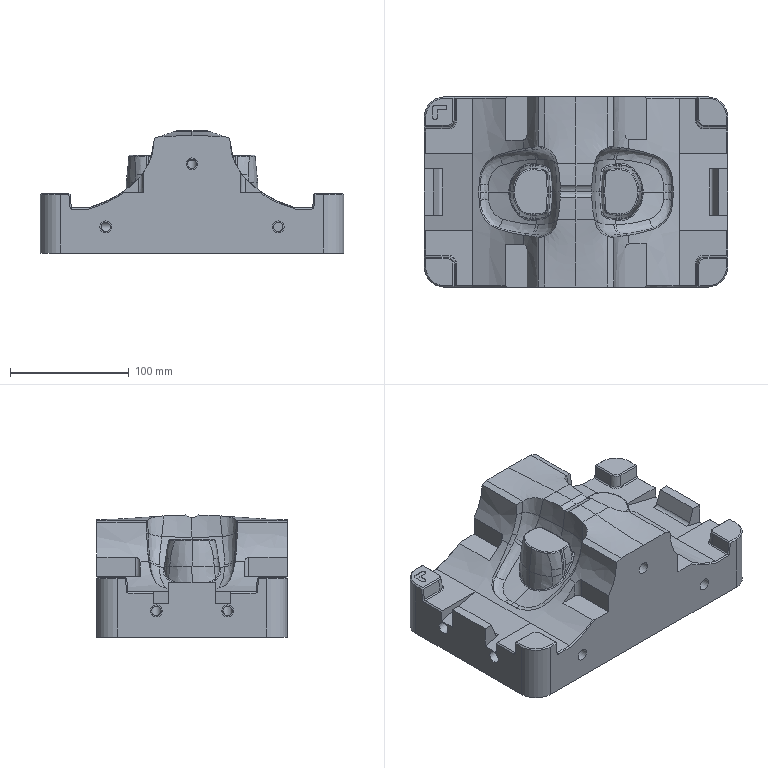NC program | NX | posted with a generic post | part box 255 x 160 x 102.619 mm
Lines 47642 to 48611 of 55104:
(ZLEVEL_PROFILE_2 , TOOL : BB6R3)
N95222 M6
N95224 G54
N95226 G17 G0 G90 X-1.967 Y96.474 S3000 M3
N95228 G43 Z51. H0
N95230 Z46.4
N95232 G94 G1 Z45.9 F1800.
N95234 X-0.764
N95236 X-0.767 Y99.474
N95238 G2 X0.026 Y100.269 R0.794
N95240 G1 X7.545
N95242 G2 X8.35 Y99.475 R0.8
N95244 G1 Y60.528
N95246 G2 X7.545 Y59.735 R0.8
N95248 G1 X0.026
N95250 G2 X-0.767 Y60.529 R0.794
N95252 G1 X-0.935 Z45.85
N95254 X-1.075 Z45.801
N95256 G3 X0.026 Y59.426 R1.102
N95258 G1 X7.545
N95260 G3 X8.659 Y60.528 R1.108
N95262 G1 Y99.475
N95264 G3 X7.545 Y100.577 R1.108
N95266 G1 X0.026
N95268 G3 X-1.075 Y99.474 R1.102
N95270 G1 X-1.197 Y99.475 Z45.751
N95272 X-1.306 Y99.476 Z45.701
N95274 G2 X0.026 Y100.807 R1.332
N95276 G1 X7.545
N95278 G2 X8.889 Y99.475 R1.338
N95280 G1 Y60.528
N95282 G2 X7.545 Y59.196 R1.338
N95284 G1 X0.026
N95286 G2 X-1.306 Y60.527 R1.332
N95288 G1 X-1.404 Z45.651
N95290 X-1.495 Z45.601
N95292 G3 X0.026 Y59.007 R1.52
N95294 G1 X7.545
N95296 G3 X9.078 Y60.528 R1.527
N95298 G1 Y99.475
N95300 G3 X7.545 Y100.996 R1.527
N95302 G1 X0.026
N95304 G3 X-1.495 Y99.476 R1.52
N95306 G1 X-1.578 Z45.551
N95308 X-1.656 Z45.502
N95310 G2 X0.026 Y101.158 R1.682
N95312 G1 X7.545
N95314 G2 X9.24 Y99.475 R1.689
N95316 G1 Y60.528
N95318 G2 X7.545 Y58.846 R1.689
N95320 G1 X0.026
N95322 G2 X-1.656 Y60.527 R1.682
N95324 G1 X-1.729 Z45.452
N95326 X-1.798 Z45.402
N95328 G3 X0.026 Y58.704 R1.823
N95330 G1 X7.545
N95332 G3 X9.381 Y60.528 R1.83
N95334 G1 Y99.475
N95336 G3 X7.545 Y101.299 R1.83
N95338 G1 X0.026
N95340 G3 X-1.798 Y99.476 R1.823
N95342 G1 X-1.924 Y99.46 Z45.302
N95344 G2 X0.026 Y101.425 R1.957
N95346 G1 X7.545
N95348 G2 X9.507 Y99.475 R1.956
N95350 G1 Y60.528
N95352 G2 X7.545 Y58.578 R1.956
N95354 G1 X0.026
N95356 G2 X-1.924 Y60.543 R1.957
N95358 G1 X-2.037 Z45.202
N95360 G3 X0.026 Y58.465 R2.071
N95362 G1 X7.545
N95364 G3 X9.62 Y60.528 R2.07
N95366 G1 Y99.475
N95368 G3 X7.545 Y101.539 R2.07
N95370 G1 X0.026
N95372 G3 X-2.037 Y99.46 R2.071
N95374 G1 X-2.14 Z45.103
N95376 G2 X0.026 Y101.641 R2.173
N95378 G1 X7.545
N95380 G2 X9.723 Y99.475 R2.172
N95382 G1 Y60.528
N95384 G2 X7.545 Y58.362 R2.172
N95386 G1 X0.026
N95388 G2 X-2.14 Y60.543 R2.173
N95390 G1 X-2.233 Z45.003
N95392 G3 X0.026 Y58.268 R2.267
N95394 G1 X7.545
N95396 G3 X9.817 Y60.528 R2.266
N95398 G1 Y99.475
N95400 G3 X7.545 Y101.735 R2.266
N95402 G1 X0.026
N95404 G3 X-2.233 Y99.46 R2.267
N95406 G1 X-2.319 Z44.903
N95408 G2 X0.026 Y101.82 R2.352
N95410 G1 X7.545
N95412 G2 X9.902 Y99.475 R2.352
N95414 G1 Y60.528
N95416 G2 X7.545 Y58.183 R2.352
N95418 G1 X0.026
N95420 G2 X-2.319 Y60.543 R2.352
N95422 G1 X-2.397 Z44.804
N95424 G3 X0.026 Y58.104 R2.431
N95426 G1 X7.545
N95428 G3 X9.981 Y60.528 R2.43
N95430 G1 Y99.475
N95432 G3 X7.545 Y101.899 R2.43
N95434 G1 X0.026
N95436 G3 X-2.397 Y99.46 R2.431
N95438 G1 X-2.469 Y99.497 Z44.704
N95440 G2 X0.062 Y101.971 R2.503
N95442 G1 X7.574
N95444 G2 X10.053 Y99.475 R2.487
N95446 G1 Y60.528
N95448 G2 X7.59 Y58.032 R2.479
N95450 G1 X0.062
N95452 G2 X-2.469 Y60.506 R2.503
N95454 G1 X-2.535 Z44.604
N95456 G3 X0. Y57.967 R2.537
N95458 G1 X7.592
N95460 G3 X10.119 Y60.528 R2.544
N95462 G1 Y99.475
N95464 G3 X7.559 Y102.037 R2.561
N95466 G1 X-0.001
N95468 G3 X-2.535 Y99.497 R2.537
N95470 G1 X-2.595 Y99.498 Z44.505
N95472 G2 X0.021 Y102.097 R2.608
N95474 G1 X7.583
N95476 G2 X10.179 Y99.475 R2.609
N95478 G1 Y60.528
N95480 G2 X7.592 Y57.906 R2.605
N95482 G1 X0.021
N95484 G2 X-2.595 Y60.505 R2.608
N95486 G1 X-2.651 Y60.504 Z44.405
N95488 G3 X0.009 Y57.851 R2.656
N95490 G1 X7.585
N95492 G3 X10.234 Y60.528 R2.664
N95494 G1 Y99.475
N95496 G3 X7.578 Y102.152 R2.667
N95498 G1 X0.009
N95500 G3 X-2.651 Y99.499 R2.656
N95502 G1 X-2.701 Y99.5 Z44.305
N95504 G2 X0.001 Y102.203 R2.703
N95506 G1 X7.578
N95508 G2 X10.196 Y100.175 R2.726
N95510 G1 X10.267 Y99.507
N95512 X10.285 Y99.475
N95514 Y60.528
N95516 X10.267 Y60.496
N95518 X10.196 Y59.828
N95520 G2 X7.602 Y57.8 R2.727
N95522 G1 X0.001
N95524 G2 X-2.701 Y60.503 R2.703
N95526 G1 X-2.747 Z44.205
N95528 G3 X0.005 Y57.754 R2.75
N95530 G1 X7.583
N95532 G3 X10.234 Y59.828 R2.741
N95534 G1 X10.31 Y60.496
N95536 X10.331 Y60.528
N95538 Y99.475
N95540 X10.31 Y99.507
N95542 X10.234 Y100.175
N95544 G3 X7.582 Y102.249 R2.741
N95546 G1 X0.
N95548 G3 X-2.747 Y99.5 R2.748
N95550 G1 X-2.789 Y99.501 Z44.106
N95552 G2 X-0.002 Y102.29 R2.788
N95554 G1 X7.54
N95556 G2 X10.353 Y99.507 R2.774
N95558 G1 X10.372 Y99.475
N95560 Y60.528
N95562 X10.353 Y60.496
N95564 G2 X7.583 Y57.713 R2.773
N95566 G1 X0.01
N95568 G2 X-2.789 Y60.502 R2.794
N95570 G1 X-2.826 Z44.006
N95572 G3 X0.003 Y57.675 R2.828
N95574 G1 X7.58
N95576 G3 X10.41 Y60.502 R2.847
N95578 G1 Y99.502
N95580 G3 X7.553 Y102.328 R2.847
N95582 G1 X0.003
N95584 G3 X-2.826 Y99.501 R2.828
N95586 G1 X-2.86 Y99.47 Z43.906
N95588 G2 X0.012 Y102.361 R2.882
N95590 G1 X7.578
N95592 G2 X10.446 Y99.502 R2.89
N95594 G1 Y60.502
N95596 G2 X7.578 Y57.642 R2.89
N95598 G1 X0.012
N95600 G2 X-2.86 Y60.534 R2.882
N95602 G1 X-2.89 Y60.533 Z43.807
N95604 G3 X0.025 Y57.612 R2.918
N95606 G1 X7.554
N95608 G3 X10.482 Y60.502 R2.909
N95610 G1 Y99.502
N95612 G3 X7.549 Y102.391 R2.912
N95614 G1 X0.025
N95616 G3 X-2.89 Y99.47 R2.918
N95618 G1 X-2.916 Z43.707
N95620 G2 X-0.001 Y102.417 R2.931
N95622 G1 X7.581
N95624 G2 X10.519 Y99.502 R2.965
N95626 G1 Y60.502
N95628 G2 X7.528 Y57.586 R2.953
N95630 G1 X0.02
N95632 G2 X-2.916 Y60.533 R2.941
N95634 G1 X-2.938 Y60.532 Z43.607
N95636 G3 X0.019 Y57.564 R2.963
N95638 G1 X7.57
N95640 G3 X10.555 Y60.502 R2.996
N95642 G1 Y99.502
N95644 G3 X7.559 Y102.439 R2.996
N95646 G1 X0.019
N95648 G3 X-2.938 Y99.471 R2.963
N95650 G1 X-2.957 Z43.508
N95652 G2 X0.001 Y102.458 R2.98
N95654 G1 X7.54
N95656 G2 X10.591 Y99.502 R3.025
N95658 G1 Y60.502
N95660 G2 X7.552 Y57.545 R3.025
N95662 G1 X0.001
N95664 G2 X-2.957 Y60.532 R2.98
N95666 G1 X-2.972 Z43.408
N95668 G3 X0.028 Y57.529 R3.018
N95670 G1 X7.579
N95672 G3 X10.628 Y60.502 R3.052
N95674 G1 Y99.502
N95676 G3 X7.567 Y102.474 R3.053
N95678 G1 X0.028
N95680 G3 X-2.972 Y99.471 R3.001
N95682 G1 X-2.984 Z43.308
N95684 G2 X0.016 Y102.486 R3.016
N95686 G1 X7.555
N95688 G2 X9.976 Y101.361 R3.218
N95690 X10.664 Y99.502 R2.857
N95692 G1 Y60.502
N95694 G2 X8.299 Y57.607 R3.047
N95696 G1 X7.567 Y57.517
N95698 X0.016
N95700 G2 X-2.974 Y60.46 R2.986
N95702 G1 X-2.984 Y60.532
N95704 X-2.993 Z43.208
N95706 G3 X0.007 Y57.509 R3.011
N95708 G1 X7.558
N95710 X7.66 Y57.515
N95712 X8.286 Y57.593
N95714 X8.387 Y57.626
N95716 X8.783 Y57.752
N95718 G3 X10.7 Y60.502 R3.021
N95720 G1 Y99.512
N95722 G3 X10.008 Y101.367 R2.831
N95724 X7.547 Y102.494 R3.27
N95726 G1 X0.007
N95728 G3 X-2.993 Y99.471 R3.011
N95730 G1 X-2.998 Z43.109
N95732 G2 X0.002 Y102.5 R3.014
N95734 G1 X7.541
N95736 G2 X10.045 Y101.366 R3.3
N95738 X10.736 Y99.518 R2.815
N95740 G1 Y60.502
N95742 G2 X9.382 Y58.048 R2.979
N95744 G1 X9.114 Y57.901
N95746 G2 X7.573 Y57.504 R3.189
N95748 G1 X0.002
N95750 G2 X-2.998 Y60.532 R3.014
N95752 G1 Y60.516 Z43.009
N95754 G3 X0. Y57.502 R3.006
N95756 G1 X7.551
N95758 G3 X8.856 Y57.752 R3.584
N95760 X10.773 Y60.502 R3.019
N95762 G1 Y99.519
N95764 G3 X10.082 Y101.365 R2.811
N95766 X7.539 Y102.502 R3.31
N95768 G1 X0.
N95770 G3 X-2.998 Y99.488 R3.006
N95772 G1 X-3. Y99.502 Z42.909
N95774 X-2.994 Y99.684
N95776 G2 X0. Y102.502 R3.
N95778 G1 X7.616
N95780 G2 X10.186 Y101.275 R3.273
N95782 X10.809 Y99.502 R2.854
N95784 G1 Y60.502
N95786 G2 X8.83 Y57.73 R3.011
N95788 X7.616 Y57.502 R3.515
N95790 G1 X0.
N95792 G2 X-2.994 Y60.309 R3.
N95794 G1 X-3. Y60.502
N95796 Z42.81
N95798 X-2.994 Y60.309
N95800 G3 X0. Y57.502 R3.
N95802 G1 X7.653
N95804 G3 X8.811 Y57.711 R3.458
N95806 G1 X8.929 Y57.752
N95808 G3 X10.845 Y60.502 R3.012
N95810 G1 Y99.502
N95812 G3 X10.158 Y101.361 R2.909
N95814 X7.653 Y102.502 R3.312
N95816 G1 X0.
N95818 G3 X-2.995 Y99.683 R3.
N95820 G1 X-3. Y99.502
N95822 Z42.71
N95824 X-2.995 Y99.681
N95826 G2 X0. Y102.502 R3.
N95828 G1 X7.689
N95830 G2 X10.194 Y101.361 R3.311
N95832 X10.882 Y99.502 R2.897
N95834 G1 Y60.502
N95836 G2 X8.965 Y57.752 R3.007
N95838 G1 X8.792 Y57.692
N95840 G2 X7.689 Y57.502 R3.547
N95842 G1 X0.
N95844 G2 X-2.994 Y60.309 R3.
N95846 G1 X-3. Y60.502
N95848 Z42.61
N95850 X-2.994 Y60.309
N95852 G3 X0. Y57.502 R3.
N95854 G1 X7.725
N95856 G3 X9.002 Y57.752 R3.816
N95858 X10.918 Y60.502 R3.009
N95860 G1 Y99.502
N95862 G3 X9.586 Y101.937 R2.95
N95864 X7.725 Y102.502 R3.415
N95866 G1 X0.
N95868 G3 X-2.995 Y99.679 R3.
N95870 G1 X-3. Y99.502
N95872 Z42.511
N95874 X-2.995 Y99.676
N95876 G2 X0. Y102.502 R3.
N95878 G1 X7.762
N95880 G2 X10.267 Y101.361 R3.304
N95882 X10.954 Y99.502 R2.889
N95884 G1 Y60.502
N95886 G2 X9.038 Y57.752 R3.008
N95888 X7.762 Y57.502 R3.853
N95890 G1 X0.
N95892 G2 X-2.994 Y60.309 R3.
N95894 G1 X-3. Y60.502
N95896 Z42.411
N95898 X-2.994 Y60.309
N95900 G3 X0. Y57.502 R3.
N95902 G1 X7.798
N95904 G3 X9.636 Y58.048 R3.39
N95906 X10.99 Y60.502 R2.967
N95908 G1 Y99.502
N95910 G3 X10.303 Y101.361 R2.904
N95912 X7.798 Y102.502 R3.289
N95914 G1 X0.
N95916 G3 X-2.995 Y99.674 R3.
N95918 G1 X-3. Y99.502
N95920 Z42.311
N95922 X-2.995 Y99.671
N95924 G2 X0. Y102.502 R3.
N95926 G1 X7.834
N95928 G2 X9.672 Y101.955 R3.458
N95930 X11.027 Y99.502 R2.969
N95932 G1 Y60.502
N95934 G2 X8.987 Y57.709 R3.006
N95936 X7.834 Y57.502 R3.803
N95938 G1 X0.
N95940 G2 X-2.994 Y60.309 R3.
N95942 G1 X-3. Y60.502
N95944 Z42.211
N95946 X-2.994 Y60.309
N95948 G3 X0. Y57.502 R3.
N95950 G1 X7.87
N95952 G3 X8.987 Y57.696 R3.859
N95954 X11.063 Y60.502 R3.006
N95956 G1 Y99.502
N95958 G3 X10.375 Y101.361 R2.899
N95960 X7.87 Y102.502 R3.31
N95962 G1 X0.
N95964 G3 X-2.995 Y99.667 R3.
N95966 G1 X-3. Y99.502
N95968 Z42.112
N95970 X-2.996 Y99.662
N95972 G2 X0. Y102.502 R3.
N95974 G1 X7.907
N95976 G2 X10.412 Y101.361 R3.307
N95978 X11.099 Y99.502 R2.897
N95980 G1 Y60.502
N95982 G2 X8.987 Y57.684 R3.008
N95984 X7.907 Y57.502 R3.894
N95986 G1 X0.
N95988 G2 X-2.994 Y60.309 R3.
N95990 G1 X-3. Y60.502
N95992 Z42.012
N95994 X-2.994 Y60.309
N95996 G3 X0. Y57.502 R3.
N95998 G1 X7.943
N96000 G3 X8.987 Y57.671 R3.897
N96002 X11.136 Y60.502 R3.012
N96004 G1 Y99.502
N96006 G3 X10.186 Y101.634 R2.912
N96008 X7.943 Y102.502 R3.329
N96010 G1 X0.
N96012 G3 X-2.996 Y99.662 R3.
N96014 G1 X-3. Y99.502
N96016 Z41.912
N96018 X-2.996 Y99.662
N96020 G2 X0. Y102.502 R3.
N96022 G1 X7.979
N96024 G2 X10.186 Y101.668 R3.332
N96026 X11.172 Y99.502 R2.923
N96028 G1 Y60.502
N96030 G2 X8.987 Y57.659 R3.018
N96032 X7.979 Y57.502 R3.854
N96034 G1 X0.
N96036 G2 X-2.994 Y60.309 R3.
N96038 G1 X-3. Y60.502
N96040 Z41.813
N96042 X-2.994 Y60.309
N96044 G3 X0. Y57.502 R3.
N96046 G1 X8.016
N96048 G3 X9.292 Y57.752 R3.643
N96050 X11.208 Y60.502 R3.01
N96052 G1 Y99.502
N96054 G3 X10.521 Y101.361 R2.905
N96056 X8.016 Y102.502 R3.293
N96058 G1 X0.
N96060 G3 X-2.996 Y99.662 R3.
N96062 G1 X-3. Y99.502
N96064 Z41.713
N96066 X-2.994 Y99.689
N96068 G2 X0. Y102.502 R3.
N96070 G1 X8.052
N96072 G2 X10.557 Y101.361 R3.296
N96074 X11.244 Y99.502 R2.891
N96076 G1 Y60.502
N96078 G2 X8.987 Y57.634 R3.035
N96080 X8.052 Y57.502 R4.166
N96082 G1 X0.
N96084 G2 X-2.994 Y60.309 R3.
N96086 G1 X-3. Y60.502
N96088 Z41.613
N96090 X-2.994 Y60.309
N96092 G3 X0. Y57.502 R3.
N96094 G1 X8.088
N96096 G3 X9.204 Y57.696 R3.624
N96098 X11.281 Y60.502 R3.007
N96100 G1 Y99.502
N96102 G3 X10.593 Y101.361 R2.897
N96104 X8.088 Y102.502 R3.31
N96106 G1 X0.
N96108 G3 X-2.994 Y99.689 R3.
N96110 G1 X-3. Y99.502
N96112 Z41.514
N96114 X-2.994 Y99.689
N96116 G2 X0. Y102.502 R3.
N96118 G1 X8.124
N96120 G2 X10.629 Y101.361 R3.318
N96122 X11.317 Y99.502 R2.901
N96124 G1 Y60.502
N96126 G2 X9.185 Y57.677 R3.015
N96128 X8.124 Y57.502 R3.807
N96130 G1 X0.
N96132 G2 X-2.994 Y60.309 R3.
N96134 G1 X-3. Y60.502
N96136 Z41.414
N96138 X-2.994 Y60.309
N96140 G3 X0. Y57.502 R3.
N96142 G1 X8.161
N96144 G3 X9.437 Y57.752 R3.881
N96146 X11.353 Y60.502 R3.016
N96148 G1 Y99.502
N96150 G3 X10.666 Y101.361 R2.9
N96152 X8.161 Y102.502 R3.32
N96154 G1 X0.
N96156 G3 X-2.994 Y99.689 R3.
N96158 G1 X-3. Y99.502
N96160 Z41.314
N96162 X-2.994 Y99.689
N96164 G2 X0. Y102.502 R3.
N96166 G1 X8.197
N96168 G2 X10.702 Y101.361 R3.306
N96170 X11.39 Y99.502 R2.898
N96172 G1 Y60.502
N96174 G2 X10.035 Y58.048 R2.966
N96176 X8.197 Y57.502 R3.407
N96178 G1 X0.
N96180 G2 X-2.994 Y60.309 R3.
N96182 G1 X-3. Y60.502
N96184 Z41.215
N96186 X-2.994 Y60.309
N96188 G3 X0. Y57.502 R3.
N96190 G1 X8.3
N96192 X8.393 Y57.508
N96194 X9.131 Y57.623
N96196 G3 X11.426 Y60.502 R3.04
N96198 G1 Y99.502
N96200 G3 X10.738 Y101.361 R2.901
N96202 X8.233 Y102.502 R3.318
N96204 G1 X0.
N96206 G3 X-2.994 Y99.689 R3.
N96208 G1 X-3. Y99.502
N96210 Z41.115
N96212 X-2.994 Y99.689
N96214 G2 X0. Y102.502 R3.
N96216 G1 X8.27
N96218 G2 X10.186 Y101.894 R3.369
N96220 X11.462 Y99.502 R2.917
N96222 G1 Y60.502
N96224 G2 X10.107 Y58.048 R2.957
N96226 X8.27 Y57.502 R3.473
N96228 G1 X0.
N96230 G2 X-2.994 Y60.309 R3.
N96232 G1 X-3. Y60.502
N96234 Z41.015
N96236 X-2.994 Y60.309
N96238 G3 X0. Y57.502 R3.
N96240 G1 X8.306
N96242 G3 X10.144 Y58.048 R3.476
N96244 X11.498 Y60.502 R2.961
N96246 G1 Y99.502
N96248 G3 X10.186 Y101.922 R2.939
N96250 X8.306 Y102.502 R3.412
N96252 G1 X0.
N96254 G3 X-2.994 Y99.689 R3.
N96256 G1 X-3. Y99.502
N96258 Z40.915
N96260 X-2.994 Y99.689
N96262 G2 X0. Y102.502 R3.
N96264 G1 X8.342
N96266 G2 X10.18 Y101.955 R3.473
N96268 X11.535 Y99.502 R2.963
N96270 G1 Y60.502
N96272 G2 X9.586 Y57.74 R3.007
N96274 X8.342 Y57.502 R3.978
N96276 G1 X0.
N96278 G2 X-2.994 Y60.309 R3.
N96280 G1 X-3. Y60.502
N96282 Z40.816
N96284 X-2.994 Y60.309
N96286 G3 X0. Y57.502 R3.
N96288 G1 X8.379
N96290 G3 X9.586 Y57.726 R3.941
N96292 X11.571 Y60.502 R3.009
N96294 G1 Y99.502
N96296 G3 X10.216 Y101.955 R2.964
N96298 X8.379 Y102.502 R3.477
N96300 G1 X0.
N96302 G3 X-2.994 Y99.689 R3.
N96304 G1 X-3. Y99.502
N96306 Z40.716
N96308 X-2.994 Y99.689
N96310 G2 X0. Y102.502 R3.
N96312 G1 X8.415
N96314 G2 X10.252 Y101.955 R3.493
N96316 X11.607 Y99.502 R2.969
N96318 G1 Y60.502
N96320 G2 X10.252 Y58.048 R2.969
N96322 X8.415 Y57.502 R3.493
N96324 G1 X0.
N96326 G2 X-2.994 Y60.309 R3.
N96328 G1 X-3. Y60.502
N96330 Z40.616
N96332 X-2.994 Y60.309
N96334 G3 X0. Y57.502 R3.
N96336 G1 X8.451
N96338 G3 X9.727 Y57.752 R3.928
N96340 X11.644 Y60.502 R3.012
N96342 G1 Y99.502
N96344 G3 X10.289 Y101.955 R2.968
N96346 X8.451 Y102.502 R3.497
N96348 G1 X0.
N96350 G3 X-2.994 Y99.689 R3.
N96352 G1 X-3. Y99.502
N96354 Z40.517
N96356 X-2.994 Y99.689
N96358 G2 X0. Y102.502 R3.
N96360 G1 X8.487
N96362 G2 X10.325 Y101.955 R3.489
N96364 X11.68 Y99.502 R2.96
N96366 G1 Y60.502
N96368 G2 X9.764 Y57.752 R3.009
N96370 X8.487 Y57.502 R3.985
N96372 G1 X0.
N96374 G2 X-2.994 Y60.309 R3.
N96376 G1 X-3. Y60.502
N96378 Z40.417
N96380 X-2.994 Y60.309
N96382 G3 X0. Y57.502 R3.
N96384 G1 X8.524
N96386 G3 X9.8 Y57.752 R3.976
N96388 X11.716 Y60.502 R3.009
N96390 G1 Y99.502
N96392 G3 X10.361 Y101.955 R2.963
N96394 X8.524 Y102.502 R3.467
N96396 G1 X0.
N96398 G3 X-2.994 Y99.689 R3.
N96400 G1 X-3. Y99.502
N96402 Z40.317
N96404 X-2.994 Y99.689
N96406 G2 X0. Y102.502 R3.
N96408 G1 X8.56
N96410 G2 X10.398 Y101.955 R3.453
N96412 X11.752 Y99.502 R2.962
N96414 G1 Y60.502
N96416 G2 X9.836 Y57.752 R3.007
N96418 X8.56 Y57.502 R3.996
N96420 G1 X0.
N96422 G2 X-2.994 Y60.309 R3.
N96424 G1 X-3. Y60.502
N96426 Z40.218
N96428 X-2.994 Y60.309
N96430 G3 X0. Y57.502 R3.
N96432 G1 X8.596
N96434 G3 X9.586 Y57.652 R4.808
N96436 X11.789 Y60.502 R3.024
N96438 G1 Y99.502
N96440 G3 X10.785 Y101.682 R2.914
N96442 X8.596 Y102.502 R3.336
N96444 G1 X0.
N96446 G3 X-2.994 Y99.689 R3.
N96448 G1 X-3. Y99.502
N96450 Z40.118
N96452 X-2.994 Y99.689
N96454 G2 X0. Y102.502 R3.
N96456 G1 X8.633
N96458 G2 X11.137 Y101.361 R3.306
N96460 X11.825 Y99.502 R2.899
N96462 G1 Y60.502
N96464 G2 X9.586 Y57.642 R3.026
N96466 X8.633 Y57.502 R4.775
N96468 G1 X0.
N96470 G2 X-2.994 Y60.309 R3.
N96472 G1 X-3. Y60.502
N96474 Z40.018
N96476 X-2.994 Y60.309
N96478 G3 X0. Y57.502 R3.
N96480 G1 X8.669
N96482 G3 X9.586 Y57.632 R4.674
N96484 X11.861 Y60.502 R3.027
N96486 G1 Y99.502
N96488 G3 X11.174 Y101.361 R2.891
N96490 X8.669 Y102.502 R3.307
N96492 G1 X0.
N96494 G3 X-2.994 Y99.689 R3.
N96496 G1 X-3. Y99.502
N96498 Z39.918
N96500 X-2.994 Y99.689
N96502 G2 X0. Y102.502 R3.
N96504 G1 X8.705
N96506 G2 X11.21 Y101.361 R3.304
N96508 X11.898 Y99.502 R2.9
N96510 G1 Y60.502
N96512 G2 X9.586 Y57.621 R3.034
N96514 X8.705 Y57.502 R4.472
N96516 G1 X0.
N96518 G2 X-2.994 Y60.309 R3.
N96520 G1 X-3. Y60.502
N96522 Z39.819
N96524 X-2.994 Y60.309
N96526 G3 X0. Y57.502 R3.
N96528 G1 X8.741
N96530 G3 X10.018 Y57.752 R3.517
N96532 X11.934 Y60.502 R3.015
N96534 G1 Y99.502
N96536 G3 X11.246 Y101.361 R2.901
N96538 X8.741 Y102.502 R3.297
N96540 G1 X0.
N96542 G3 X-2.994 Y99.689 R3.
N96544 G1 X-3. Y99.502
N96546 Z39.719
N96548 X-2.994 Y99.689
N96550 G2 X0. Y102.502 R3.
N96552 G1 X8.778
N96554 G2 X11.283 Y101.361 R3.297
N96556 X11.97 Y99.502 R2.898
N96558 G1 Y60.502
N96560 G2 X9.586 Y57.601 R3.046
N96562 X8.778 Y57.502 R3.962
N96564 G1 X0.
N96566 G2 X-2.994 Y60.309 R3.
N96568 G1 X-3. Y60.502
N96570 Z39.619
N96572 X-2.994 Y60.309
N96574 G3 X0. Y57.502 R3.
N96576 G1 X8.814
N96578 G3 X10.09 Y57.752 R3.422
N96580 X12.006 Y60.502 R3.014
N96582 G1 Y99.552
N96584 G3 X11.708 Y100.768 R2.627
N96586 X8.814 Y102.502 R3.228
N96588 G1 X0.
N96590 G3 X-2.994 Y99.689 R3.
N96592 G1 X-3. Y99.502
N96594 Z39.52
N96596 X-2.994 Y99.689
N96598 G2 X0. Y102.502 R3.
N96600 G1 X8.85
N96602 G2 X11.384 Y101.322 R3.279
N96604 X12.043 Y99.502 R2.875
N96606 G1 Y60.502
N96608 G2 X10.047 Y57.724 R3.01
N96610 X8.85 Y57.502 R3.366
N96612 G1 X0.
N96614 G2 X-2.994 Y60.309 R3.
N96616 G1 X-3. Y60.502
N96618 Z39.42
N96620 X-2.994 Y60.309
N96622 G3 X0. Y57.502 R3.
N96624 G1 X8.887
N96626 G3 X11.097 Y58.337 R3.379
N96628 X12.079 Y60.5 R2.874
N96630 G1 Y99.502
N96632 G3 X11.391 Y101.361 R2.895
N96634 X8.887 Y102.502 R3.301
N96636 G1 X0.
N96638 G3 X-2.994 Y99.689 R3.
N96640 G1 X-3. Y99.502
N96642 Z39.32
N96644 X-2.994 Y99.689
N96646 G2 X0. Y102.502 R3.
N96648 G1 X8.923
N96650 G2 X11.428 Y101.361 R3.3
N96652 X12.115 Y99.502 R2.906
N96654 G1 Y60.501
N96656 G2 X10.898 Y58.141 R2.895
N96658 X8.923 Y57.502 R3.458
N96660 G1 X0.
N96662 G2 X-2.997 Y60.347 R3.001
N96664 G1 X-3. Y60.502
N96666 Z39.221
N96668 X-2.994 Y60.309
N96670 G3 X0. Y57.502 R3.
N96672 G1 X8.959
N96674 G3 X10.235 Y57.752 R3.733
N96676 X12.152 Y60.502 R3.008
N96678 G1 Y99.502
N96680 G3 X11.464 Y101.361 R2.891
N96682 X8.959 Y102.502 R3.299
N96684 G1 X0.
N96686 G3 X-2.994 Y99.689 R3.
N96688 G1 X-3. Y99.502
N96690 Z39.121
N96692 X-2.994 Y99.689
N96694 G2 X0. Y102.502 R3.
N96696 G1 X8.995
N96698 G2 X11.5 Y101.361 R3.3
N96700 X12.188 Y99.502 R2.903
N96702 G1 Y60.502
N96704 G2 X10.272 Y57.752 R3.011
N96706 X8.995 Y57.502 R3.751
N96708 G1 X0.
N96710 G2 X-2.997 Y60.347 R3.001
N96712 G1 X-3. Y60.502
N96714 Z39.021
N96716 X-2.994 Y60.309
N96718 G3 X0. Y57.502 R3.
N96720 G1 X9.032
N96722 G3 X10.869 Y58.048 R3.37
N96724 X12.224 Y60.502 R2.969
N96726 G1 Y99.549
N96728 G3 X11.926 Y100.768 R2.64
N96730 X9.032 Y102.502 R3.222
N96732 G1 X0.
N96734 G3 X-2.994 Y99.689 R3.
N96736 G1 X-3. Y99.502
N96738 Z38.921
N96740 X-2.994 Y99.689
N96742 G2 X0. Y102.502 R3.
N96744 G1 X9.068
N96746 G2 X11.573 Y101.361 R3.296
N96748 X12.26 Y99.502 R2.9
N96750 G1 Y60.502
N96752 G2 X10.344 Y57.752 R3.011
N96754 G1 X10.186 Y57.697
N96756 G2 X9.068 Y57.502 R3.484
N96758 G1 X0.
N96760 G2 X-2.997 Y60.347 R3.001
N96762 G1 X-3. Y60.502
N96764 Z38.822
N96766 X-2.994 Y60.309
N96768 G3 X0. Y57.502 R3.
N96770 G1 X9.104
N96772 G3 X10.186 Y57.684 R3.516
N96774 G1 X10.38 Y57.752
N96776 G3 X12.297 Y60.502 R3.009
N96778 G1 Y99.502
N96780 G3 X11.609 Y101.361 R2.896
N96782 X9.104 Y102.502 R3.296
N96784 G1 X0.
N96786 G3 X-2.994 Y99.689 R3.
N96788 G1 X-3. Y99.502
N96790 Z38.722
N96792 X-2.994 Y99.689
N96794 G2 X0. Y102.502 R3.
N96796 G1 X9.141
N96798 G2 X11.645 Y101.361 R3.292
N96800 X12.333 Y99.502 R2.908
N96802 G1 Y60.502
N96804 G2 X10.417 Y57.752 R3.009
N96806 X9.141 Y57.502 R3.633
N96808 G1 X0.
N96810 G2 X-2.997 Y60.347 R3.001
N96812 G1 X-3. Y60.502
N96814 Z38.622
N96816 X-2.994 Y60.309
N96818 G3 X0. Y57.502 R3.
N96820 G1 X9.177
N96822 G3 X10.453 Y57.752 R3.569
N96824 X12.369 Y60.502 R3.009
N96826 G1 Y99.502
N96828 G3 X11.682 Y101.361 R2.91
N96830 X9.177 Y102.502 R3.286
N96832 G1 X0.
N96834 G3 X-2.994 Y99.689 R3.
N96836 G1 X-3. Y99.502
N96838 Z38.523
N96840 X-2.994 Y99.689
N96842 G2 X0. Y102.502 R3.
N96844 G1 X9.213
N96846 G2 X11.718 Y101.361 R3.292
N96848 X12.406 Y99.502 R2.906
N96850 G1 Y60.502
N96852 G2 X10.186 Y57.647 R3.026
N96854 X9.213 Y57.502 R3.781
N96856 G1 X0.
N96858 G2 X-2.997 Y60.347 R3.001
N96860 G1 X-3. Y60.502
N96862 Z38.423
N96864 X-2.994 Y60.309
N96866 G3 X0. Y57.502 R3.
N96868 G1 X9.249
N96870 G3 X10.526 Y57.752 R3.446
N96872 X12.442 Y60.502 R3.009
N96874 G1 Y99.502
N96876 G3 X11.754 Y101.361 R2.895
N96878 X9.249 Y102.502 R3.287
N96880 G1 X0.
N96882 G3 X-2.994 Y99.689 R3.
N96884 G1 X-3. Y99.502
N96886 Z38.323
N96888 X-2.994 Y99.689
N96890 G2 X0. Y102.502 R3.
N96892 G1 X9.286
N96894 G2 X11.791 Y101.361 R3.306
N96896 X12.478 Y99.502 R2.897
N96898 G1 Y60.502
N96900 G2 X10.562 Y57.752 R3.012
N96902 G1 X10.439 Y57.709
N96904 G2 X9.286 Y57.502 R3.523
N96906 G1 X0.
N96908 G2 X-2.997 Y60.347 R3.001
N96910 G1 X-3. Y60.502
N96912 Z38.224
N96914 X-2.994 Y60.309
N96916 G3 X0. Y57.502 R3.
N96918 G1 X9.322
N96920 G3 X10.42 Y57.69 R3.665
N96922 X12.514 Y60.502 R3.011
N96924 G1 Y99.502
N96926 G3 X11.827 Y101.361 R2.901
N96928 X9.322 Y102.502 R3.316
N96930 G1 X0.
N96932 G3 X-2.994 Y99.689 R3.
N96934 G1 X-3. Y99.502
N96936 Z38.124
N96938 X-2.994 Y99.689
N96940 G2 X0. Y102.502 R3.
N96942 G1 X9.358
N96944 G2 X11.863 Y101.361 R3.323
N96946 X12.551 Y99.502 R2.9
N96948 G1 Y60.502
N96950 G2 X10.401 Y57.671 R3.018
N96952 X9.358 Y57.502 R3.866
N96954 G1 X0.
N96956 G2 X-2.997 Y60.347 R3.001
N96958 G1 X-3. Y60.502
N96960 Z38.024
N96962 X-2.994 Y60.309
N96964 G3 X0. Y57.502 R3.
N96966 G1 X9.395
N96968 G3 X10.186 Y57.607 R3.408
N96970 G1 X10.382 Y57.652
N96972 G3 X12.587 Y60.502 R3.027
N96974 G1 Y99.502
N96976 G3 X11.9 Y101.361 R2.898
N96978 X9.395 Y102.502 R3.322
N96980 G1 X0.
N96982 G3 X-2.994 Y99.689 R3.
N96984 G1 X-3. Y99.502
N96986 Z37.924
N96988 X-2.994 Y99.689
N96990 G2 X0. Y102.502 R3.
N96992 G1 X9.431
N96994 G2 X11.936 Y101.361 R3.319
N96996 X12.623 Y99.502 R2.901
N96998 G1 Y60.502
N97000 G2 X10.363 Y57.633 R3.038
N97002 G1 X9.812 Y57.534
N97004 G2 X9.445 Y57.502 R2.079
N97006 G1 X0.
N97008 G2 X-2.997 Y60.347 R3.001
N97010 G1 X-3. Y60.502
N97012 Z37.825
N97014 X-2.994 Y60.309
N97016 G3 X0. Y57.502 R3.
N97018 G1 X9.467
N97020 X9.586 Y57.505
N97022 X10.186 Y57.595
N97024 G3 X12.66 Y60.502 R3.01
N97026 G1 Y99.502
N97028 G3 X11.384 Y101.893 R2.917
N97030 X9.467 Y102.502 R3.367
N97032 G1 X0.
N97034 G3 X-2.994 Y99.689 R3.
N97036 G1 X-3. Y99.502
N97038 Z37.725
N97040 X-2.994 Y99.689
N97042 G2 X0. Y102.502 R3.
N97044 G1 X9.503
N97046 G2 X11.384 Y101.921 R3.414
N97048 X12.696 Y99.502 R2.938
N97050 G1 Y60.502
N97052 G2 X11.341 Y58.048 R2.961
N97054 X9.503 Y57.502 R3.479
N97056 G1 X0.
N97058 G2 X-2.997 Y60.347 R3.001
N97060 G1 X-3. Y60.502
N97062 Z37.625
N97064 X-2.994 Y60.309
N97066 G3 X0. Y57.502 R3.
N97068 G1 X9.54
N97070 G3 X10.785 Y57.741 R3.997
N97072 X12.732 Y60.502 R3.006
N97074 G1 Y99.502
N97076 G3 X11.377 Y101.955 R2.963
N97078 X9.54 Y102.502 R3.482
N97080 G1 X0.
N97082 G3 X-2.994 Y99.689 R3.
N97084 G1 X-3. Y99.502
N97086 Z37.526
N97088 X-2.994 Y99.689
N97090 G2 X0. Y102.502 R3.
N97092 G1 X9.576
N97094 G2 X11.414 Y101.955 R3.477
N97096 X12.768 Y99.502 R2.964
N97098 G1 Y60.502
N97100 G2 X10.785 Y57.728 R3.006
N97102 X9.576 Y57.502 R3.961
N97104 G1 X0.
N97106 G2 X-2.997 Y60.347 R3.001
N97108 G1 X-3. Y60.502
N97110 Z37.426
N97112 X-2.994 Y60.309
N97114 G3 X0. Y57.502 R3.
N97116 G1 X9.612
N97118 G3 X10.785 Y57.715 R3.896
N97120 X12.805 Y60.502 R3.009
N97122 G1 Y99.502
N97124 G3 X11.45 Y101.955 R2.969
N97126 X9.612 Y102.502 R3.491
N97128 G1 X0.
N97130 G3 X-2.994 Y99.689 R3.
N97132 G1 X-3. Y99.502
N97134 Z37.326
N97136 X-2.994 Y99.689
N97138 G2 X0. Y102.502 R3.
N97140 G1 X9.649
N97142 G2 X11.486 Y101.955 R3.496
N97144 X12.841 Y99.502 R2.968
N97146 G1 Y60.502
N97148 G2 X10.785 Y57.702 R3.011
N97150 X9.649 Y57.502 R3.893
N97152 G1 X0.
N97154 G2 X-2.997 Y60.347 R3.001